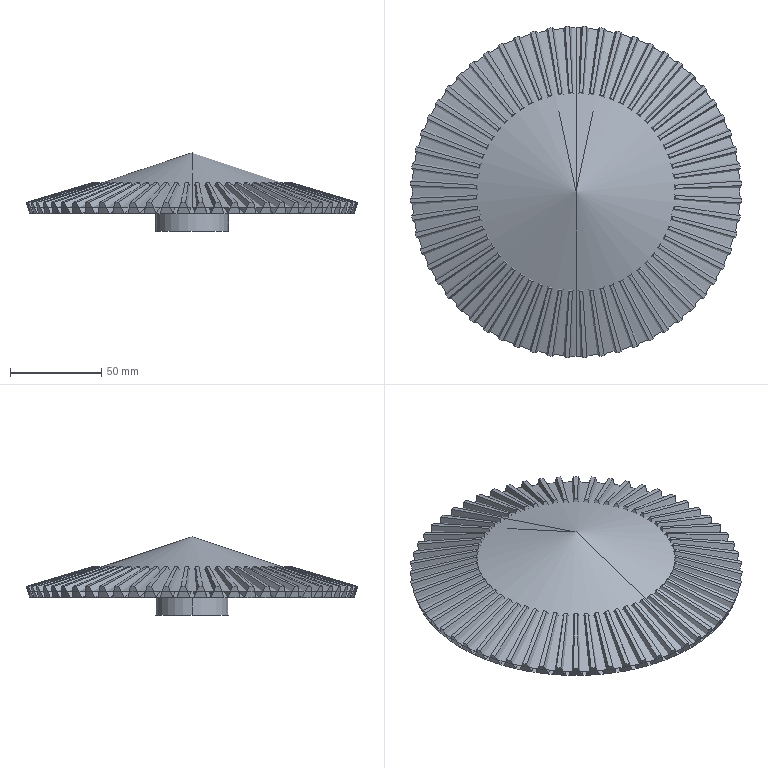Part | SolidWorks | 1 solid | 371 faces | box 181.762 x 181.762 x 42.996 mm | volume 60208 mm3 | cone 243 | spline 120 | plane 4 | cylinder 4 | commonest cylinder face diameters 30 x2 40 x2